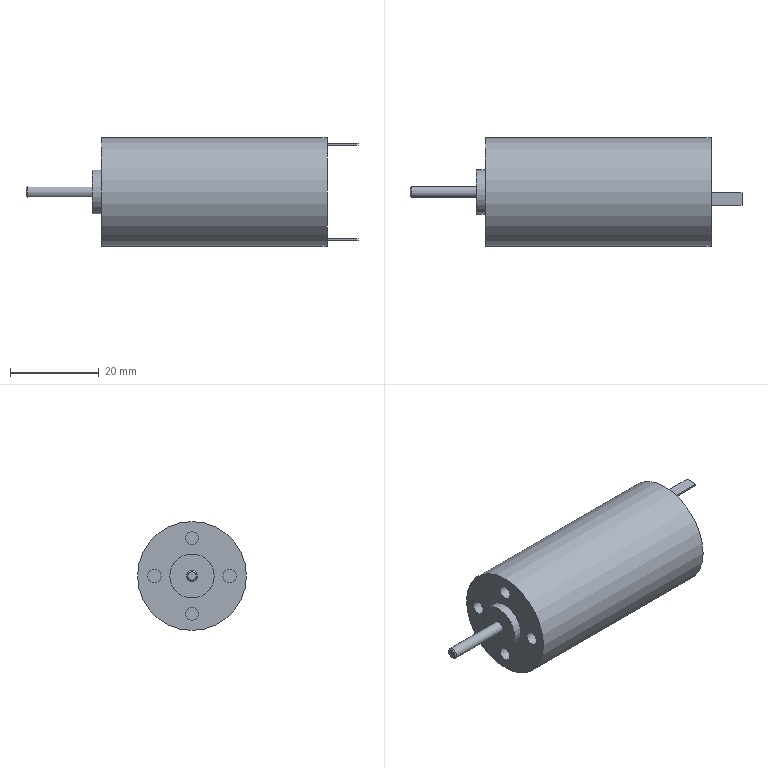Part | STEP file | Wytnij-wyci_gni_cie1_4 | 1 solid | 26 faces | box 75 x 24.6 x 24.6 mm | volume 24401 mm3 | plane 18 | cylinder 7 | cone 1 | commonest cylinder face diameters 3 x4 2.5 x1 10 x1 24.6 x1
STEP:
#1=CARTESIAN_POINT('',(0.,0.,0.));
#2=DIRECTION('',(0.,0.,1.));
#3=DIRECTION('',(1.,0.,0.));
#4=AXIS2_PLACEMENT_3D('',#1,#2,#3);
#5=CARTESIAN_POINT('',(-12.682,75.838,-107.798));
#6=VERTEX_POINT('',#5);
#7=CARTESIAN_POINT('',(38.318,75.838,-107.798));
#8=VERTEX_POINT('',#7);
#9=CARTESIAN_POINT('',(-12.682,75.838,-107.798));
#10=DIRECTION('',(1.,0.,0.));
#11=VECTOR('',#10,1.);
#12=LINE('',#9,#11);
#13=CARTESIAN_POINT('',(38.318,88.138,-107.798));
#14=DIRECTION('',(-1.,0.,0.));
#15=DIRECTION('',(0.,-1.,0.));
#16=AXIS2_PLACEMENT_3D('',#13,#14,#15);
#17=CYLINDRICAL_SURFACE('',#16,12.3);
#18=CARTESIAN_POINT('',(0.,51.));
#19=DIRECTION('',(0.,-1.));
#20=VECTOR('',#19,1.);
#21=LINE('',#18,#20);
#22=(GEOMETRIC_REPRESENTATION_CONTEXT(2)PARAMETRIC_REPRESENTATION_CONTEXT()REPRESENTATION_CONTEXT('',''));
#23=DEFINITIONAL_REPRESENTATION('',(#21),#22);
#24=PCURVE('',#17,#23);
#25=CARTESIAN_POINT('',(6.283,51.));
#26=DIRECTION('',(0.,-1.));
#27=VECTOR('',#26,1.);
#28=LINE('',#25,#27);
#29=(GEOMETRIC_REPRESENTATION_CONTEXT(2)PARAMETRIC_REPRESENTATION_CONTEXT()REPRESENTATION_CONTEXT('',''));
#30=DEFINITIONAL_REPRESENTATION('',(#28),#29);
#31=PCURVE('',#17,#30);
#32=SEAM_CURVE('',#12,(#24,#31),.PCURVE_S1.);
#33=EDGE_CURVE('',#6,#8,#32,.T.);
#34=ORIENTED_EDGE('',*,*,#33,.T.);
#35=CARTESIAN_POINT('',(38.318,88.138,-107.798));
#36=DIRECTION('',(-1.,0.,0.));
#37=DIRECTION('',(0.,-1.,0.));
#38=AXIS2_PLACEMENT_3D('',#35,#36,#37);
#39=CIRCLE('',#38,12.3);
#40=CARTESIAN_POINT('',(0.,0.));
#41=DIRECTION('',(1.,0.));
#42=VECTOR('',#41,1.);
#43=LINE('',#40,#42);
#44=(GEOMETRIC_REPRESENTATION_CONTEXT(2)PARAMETRIC_REPRESENTATION_CONTEXT()REPRESENTATION_CONTEXT('',''));
#45=DEFINITIONAL_REPRESENTATION('',(#43),#44);
#46=PCURVE('',#17,#45);
#47=CARTESIAN_POINT('',(38.318,88.138,-107.798));
#48=DIRECTION('',(1.,0.,0.));
#49=DIRECTION('',(0.,1.,0.));
#50=AXIS2_PLACEMENT_3D('',#47,#48,#49);
#51=PLANE('',#50);
#52=CARTESIAN_POINT('',(-12.3,0.));
#53=CARTESIAN_POINT('',(-12.3,21.304));
#54=CARTESIAN_POINT('',(6.15,10.652));
#55=CARTESIAN_POINT('',(24.6,0.));
#56=CARTESIAN_POINT('',(6.15,-10.652));
#57=CARTESIAN_POINT('',(-12.3,-21.304));
#58=CARTESIAN_POINT('',(-12.3,0.));
#59=(BOUNDED_CURVE()B_SPLINE_CURVE(2,(#52,#53,#54,#55,#56,#57,#58),.UNSPECIFIED.,.T.,.F.)B_SPLINE_CURVE_WITH_KNOTS((1,2,2,2,2,1),(-2.094,0.,2.094,4.189,6.283,8.378),.UNSPECIFIED.)CURVE()GEOMETRIC_REPRESENTATION_ITEM()RATIONAL_B_SPLINE_CURVE((1.,0.5,1.,0.5,1.,0.5,1.))REPRESENTATION_ITEM(''));
#60=(GEOMETRIC_REPRESENTATION_CONTEXT(2)PARAMETRIC_REPRESENTATION_CONTEXT()REPRESENTATION_CONTEXT('',''));
#61=DEFINITIONAL_REPRESENTATION('',(#59),#60);
#62=PCURVE('',#51,#61);
#63=SURFACE_CURVE('',#39,(#46,#62),.PCURVE_S1.);
#64=EDGE_CURVE('',#8,#8,#63,.T.);
#65=ORIENTED_EDGE('',*,*,#64,.T.);
#66=ORIENTED_EDGE('',*,*,#33,.F.);
#67=CARTESIAN_POINT('',(-12.682,88.138,-107.798));
#68=DIRECTION('',(1.,0.,0.));
#69=DIRECTION('',(0.,-1.,0.));
#70=AXIS2_PLACEMENT_3D('',#67,#68,#69);
#71=CIRCLE('',#70,12.3);
#72=CARTESIAN_POINT('',(6.283,51.));
#73=DIRECTION('',(-1.,0.));
#74=VECTOR('',#73,1.);
#75=LINE('',#72,#74);
#76=(GEOMETRIC_REPRESENTATION_CONTEXT(2)PARAMETRIC_REPRESENTATION_CONTEXT()REPRESENTATION_CONTEXT('',''));
#77=DEFINITIONAL_REPRESENTATION('',(#75),#76);
#78=PCURVE('',#17,#77);
#79=CARTESIAN_POINT('',(-12.682,88.138,-107.798));
#80=DIRECTION('',(-1.,0.,0.));
#81=DIRECTION('',(0.,-1.,0.));
#82=AXIS2_PLACEMENT_3D('',#79,#80,#81);
#83=PLANE('',#82);
#84=CARTESIAN_POINT('',(12.3,0.));
#85=CARTESIAN_POINT('',(12.3,-21.304));
#86=CARTESIAN_POINT('',(-6.15,-10.652));
#87=CARTESIAN_POINT('',(-24.6,0.));
#88=CARTESIAN_POINT('',(-6.15,10.652));
#89=CARTESIAN_POINT('',(12.3,21.304));
#90=CARTESIAN_POINT('',(12.3,0.));
#91=(BOUNDED_CURVE()B_SPLINE_CURVE(2,(#84,#85,#86,#87,#88,#89,#90),.UNSPECIFIED.,.T.,.F.)B_SPLINE_CURVE_WITH_KNOTS((1,2,2,2,2,1),(-2.094,0.,2.094,4.189,6.283,8.378),.UNSPECIFIED.)CURVE()GEOMETRIC_REPRESENTATION_ITEM()RATIONAL_B_SPLINE_CURVE((1.,0.5,1.,0.5,1.,0.5,1.))REPRESENTATION_ITEM(''));
#92=(GEOMETRIC_REPRESENTATION_CONTEXT(2)PARAMETRIC_REPRESENTATION_CONTEXT()REPRESENTATION_CONTEXT('',''));
#93=DEFINITIONAL_REPRESENTATION('',(#91),#92);
#94=PCURVE('',#83,#93);
#95=SURFACE_CURVE('',#71,(#78,#94),.PCURVE_S1.);
#96=EDGE_CURVE('',#6,#6,#95,.T.);
#97=ORIENTED_EDGE('',*,*,#96,.T.);
#98=EDGE_LOOP('',(#34,#65,#66,#97));
#99=FACE_BOUND('',#98,.T.);
#100=ADVANCED_FACE('',(#99),#17,.T.);
#101=CARTESIAN_POINT('',(-9.682,86.638,-99.298));
#102=VERTEX_POINT('',#101);
#103=CARTESIAN_POINT('',(-9.682,88.138,-99.298));
#104=DIRECTION('',(-1.,0.,0.));
#105=DIRECTION('',(0.,-1.,0.));
#106=AXIS2_PLACEMENT_3D('',#103,#104,#105);
#107=CIRCLE('',#106,1.5);
#108=CARTESIAN_POINT('',(-9.682,88.138,-99.298));
#109=DIRECTION('',(-1.,0.,0.));
#110=DIRECTION('',(0.,-1.,0.));
#111=AXIS2_PLACEMENT_3D('',#108,#109,#110);
#112=CYLINDRICAL_SURFACE('',#111,1.5);
#113=CARTESIAN_POINT('',(0.,0.));
#114=DIRECTION('',(1.,0.));
#115=VECTOR('',#114,1.);
#116=LINE('',#113,#115);
#117=(GEOMETRIC_REPRESENTATION_CONTEXT(2)PARAMETRIC_REPRESENTATION_CONTEXT()REPRESENTATION_CONTEXT('',''));
#118=DEFINITIONAL_REPRESENTATION('',(#116),#117);
#119=PCURVE('',#112,#118);
#120=CARTESIAN_POINT('',(-9.682,88.138,-99.298));
#121=DIRECTION('',(-1.,0.,0.));
#122=DIRECTION('',(0.,-1.,0.));
#123=AXIS2_PLACEMENT_3D('',#120,#121,#122);
#124=PLANE('',#123);
#125=CARTESIAN_POINT('',(0.,0.));
#126=DIRECTION('',(1.,0.));
#127=AXIS2_PLACEMENT_2D('',#125,#126);
#128=CIRCLE('',#127,1.5);
#129=(GEOMETRIC_REPRESENTATION_CONTEXT(2)PARAMETRIC_REPRESENTATION_CONTEXT()REPRESENTATION_CONTEXT('',''));
#130=DEFINITIONAL_REPRESENTATION('',(#128),#129);
#131=PCURVE('',#124,#130);
#132=SURFACE_CURVE('',#107,(#119,#131),.PCURVE_S1.);
#133=EDGE_CURVE('',#102,#102,#132,.T.);
#134=ORIENTED_EDGE('',*,*,#133,.T.);
#135=CARTESIAN_POINT('',(-12.682,86.638,-99.298));
#136=VERTEX_POINT('',#135);
#137=CARTESIAN_POINT('',(-12.682,86.638,-99.298));
#138=DIRECTION('',(1.,0.,0.));
#139=VECTOR('',#138,1.);
#140=LINE('',#137,#139);
#141=CARTESIAN_POINT('',(6.283,3.));
#142=DIRECTION('',(0.,-1.));
#143=VECTOR('',#142,1.);
#144=LINE('',#141,#143);
#145=(GEOMETRIC_REPRESENTATION_CONTEXT(2)PARAMETRIC_REPRESENTATION_CONTEXT()REPRESENTATION_CONTEXT('',''));
#146=DEFINITIONAL_REPRESENTATION('',(#144),#145);
#147=PCURVE('',#112,#146);
#148=CARTESIAN_POINT('',(0.,3.));
#149=DIRECTION('',(0.,-1.));
#150=VECTOR('',#149,1.);
#151=LINE('',#148,#150);
#152=(GEOMETRIC_REPRESENTATION_CONTEXT(2)PARAMETRIC_REPRESENTATION_CONTEXT()REPRESENTATION_CONTEXT('',''));
#153=DEFINITIONAL_REPRESENTATION('',(#151),#152);
#154=PCURVE('',#112,#153);
#155=SEAM_CURVE('',#140,(#147,#154),.PCURVE_S1.);
#156=EDGE_CURVE('',#136,#102,#155,.T.);
#157=ORIENTED_EDGE('',*,*,#156,.F.);
#158=CARTESIAN_POINT('',(-12.682,88.138,-99.298));
#159=DIRECTION('',(1.,0.,0.));
#160=DIRECTION('',(0.,-1.,0.));
#161=AXIS2_PLACEMENT_3D('',#158,#159,#160);
#162=CIRCLE('',#161,1.5);
#163=CARTESIAN_POINT('',(6.283,3.));
#164=DIRECTION('',(-1.,0.));
#165=VECTOR('',#164,1.);
#166=LINE('',#163,#165);
#167=(GEOMETRIC_REPRESENTATION_CONTEXT(2)PARAMETRIC_REPRESENTATION_CONTEXT()REPRESENTATION_CONTEXT('',''));
#168=DEFINITIONAL_REPRESENTATION('',(#166),#167);
#169=PCURVE('',#112,#168);
#170=CARTESIAN_POINT('',(1.5,8.5));
#171=CARTESIAN_POINT('',(1.5,5.902));
#172=CARTESIAN_POINT('',(-0.75,7.201));
#173=CARTESIAN_POINT('',(-3.,8.5));
#174=CARTESIAN_POINT('',(-0.75,9.799));
#175=CARTESIAN_POINT('',(1.5,11.098));
#176=CARTESIAN_POINT('',(1.5,8.5));
#177=(BOUNDED_CURVE()B_SPLINE_CURVE(2,(#170,#171,#172,#173,#174,#175,#176),.UNSPECIFIED.,.T.,.F.)B_SPLINE_CURVE_WITH_KNOTS((1,2,2,2,2,1),(-2.094,0.,2.094,4.189,6.283,8.378),.UNSPECIFIED.)CURVE()GEOMETRIC_REPRESENTATION_ITEM()RATIONAL_B_SPLINE_CURVE((1.,0.5,1.,0.5,1.,0.5,1.))REPRESENTATION_ITEM(''));
#178=(GEOMETRIC_REPRESENTATION_CONTEXT(2)PARAMETRIC_REPRESENTATION_CONTEXT()REPRESENTATION_CONTEXT('',''));
#179=DEFINITIONAL_REPRESENTATION('',(#177),#178);
#180=PCURVE('',#83,#179);
#181=SURFACE_CURVE('',#162,(#169,#180),.PCURVE_S1.);
#182=EDGE_CURVE('',#136,#136,#181,.T.);
#183=ORIENTED_EDGE('',*,*,#182,.T.);
#184=ORIENTED_EDGE('',*,*,#156,.T.);
#185=EDGE_LOOP('',(#134,#157,#183,#184));
#186=FACE_BOUND('',#185,.F.);
#187=ADVANCED_FACE('',(#186),#112,.F.);
#188=CARTESIAN_POINT('',(-9.682,78.138,-107.798));
#189=VERTEX_POINT('',#188);
#190=CARTESIAN_POINT('',(-9.682,79.638,-107.798));
#191=DIRECTION('',(-1.,0.,0.));
#192=DIRECTION('',(0.,-1.,0.));
#193=AXIS2_PLACEMENT_3D('',#190,#191,#192);
#194=CIRCLE('',#193,1.5);
#195=CARTESIAN_POINT('',(-9.682,79.638,-107.798));
#196=DIRECTION('',(-1.,0.,0.));
#197=DIRECTION('',(0.,-1.,0.));
#198=AXIS2_PLACEMENT_3D('',#195,#196,#197);
#199=CYLINDRICAL_SURFACE('',#198,1.5);
#200=CARTESIAN_POINT('',(0.,0.));
#201=DIRECTION('',(1.,0.));
#202=VECTOR('',#201,1.);
#203=LINE('',#200,#202);
#204=(GEOMETRIC_REPRESENTATION_CONTEXT(2)PARAMETRIC_REPRESENTATION_CONTEXT()REPRESENTATION_CONTEXT('',''));
#205=DEFINITIONAL_REPRESENTATION('',(#203),#204);
#206=PCURVE('',#199,#205);
#207=CARTESIAN_POINT('',(-9.682,79.638,-107.798));
#208=DIRECTION('',(-1.,0.,0.));
#209=DIRECTION('',(0.,-1.,0.));
#210=AXIS2_PLACEMENT_3D('',#207,#208,#209);
#211=PLANE('',#210);
#212=CARTESIAN_POINT('',(0.,0.));
#213=DIRECTION('',(1.,0.));
#214=AXIS2_PLACEMENT_2D('',#212,#213);
#215=CIRCLE('',#214,1.5);
#216=(GEOMETRIC_REPRESENTATION_CONTEXT(2)PARAMETRIC_REPRESENTATION_CONTEXT()REPRESENTATION_CONTEXT('',''));
#217=DEFINITIONAL_REPRESENTATION('',(#215),#216);
#218=PCURVE('',#211,#217);
#219=SURFACE_CURVE('',#194,(#206,#218),.PCURVE_S1.);
#220=EDGE_CURVE('',#189,#189,#219,.T.);
#221=ORIENTED_EDGE('',*,*,#220,.T.);
#222=CARTESIAN_POINT('',(-12.682,78.138,-107.798));
#223=VERTEX_POINT('',#222);
#224=CARTESIAN_POINT('',(-12.682,78.138,-107.798));
#225=DIRECTION('',(1.,0.,0.));
#226=VECTOR('',#225,1.);
#227=LINE('',#224,#226);
#228=CARTESIAN_POINT('',(6.283,3.));
#229=DIRECTION('',(0.,-1.));
#230=VECTOR('',#229,1.);
#231=LINE('',#228,#230);
#232=(GEOMETRIC_REPRESENTATION_CONTEXT(2)PARAMETRIC_REPRESENTATION_CONTEXT()REPRESENTATION_CONTEXT('',''));
#233=DEFINITIONAL_REPRESENTATION('',(#231),#232);
#234=PCURVE('',#199,#233);
#235=CARTESIAN_POINT('',(0.,3.));
#236=DIRECTION('',(0.,-1.));
#237=VECTOR('',#236,1.);
#238=LINE('',#235,#237);
#239=(GEOMETRIC_REPRESENTATION_CONTEXT(2)PARAMETRIC_REPRESENTATION_CONTEXT()REPRESENTATION_CONTEXT('',''));
#240=DEFINITIONAL_REPRESENTATION('',(#238),#239);
#241=PCURVE('',#199,#240);
#242=SEAM_CURVE('',#227,(#234,#241),.PCURVE_S1.);
#243=EDGE_CURVE('',#223,#189,#242,.T.);
#244=ORIENTED_EDGE('',*,*,#243,.F.);
#245=CARTESIAN_POINT('',(-12.682,79.638,-107.798));
#246=DIRECTION('',(1.,0.,0.));
#247=DIRECTION('',(0.,-1.,0.));
#248=AXIS2_PLACEMENT_3D('',#245,#246,#247);
#249=CIRCLE('',#248,1.5);
#250=CARTESIAN_POINT('',(6.283,3.));
#251=DIRECTION('',(-1.,0.));
#252=VECTOR('',#251,1.);
#253=LINE('',#250,#252);
#254=(GEOMETRIC_REPRESENTATION_CONTEXT(2)PARAMETRIC_REPRESENTATION_CONTEXT()REPRESENTATION_CONTEXT('',''));
#255=DEFINITIONAL_REPRESENTATION('',(#253),#254);
#256=PCURVE('',#199,#255);
#257=CARTESIAN_POINT('',(10.,0.));
#258=CARTESIAN_POINT('',(10.,-2.598));
#259=CARTESIAN_POINT('',(7.75,-1.299));
#260=CARTESIAN_POINT('',(5.5,0.));
#261=CARTESIAN_POINT('',(7.75,1.299));
#262=CARTESIAN_POINT('',(10.,2.598));
#263=CARTESIAN_POINT('',(10.,0.));
#264=(BOUNDED_CURVE()B_SPLINE_CURVE(2,(#257,#258,#259,#260,#261,#262,#263),.UNSPECIFIED.,.T.,.F.)B_SPLINE_CURVE_WITH_KNOTS((1,2,2,2,2,1),(-2.094,0.,2.094,4.189,6.283,8.378),.UNSPECIFIED.)CURVE()GEOMETRIC_REPRESENTATION_ITEM()RATIONAL_B_SPLINE_CURVE((1.,0.5,1.,0.5,1.,0.5,1.))REPRESENTATION_ITEM(''));
#265=(GEOMETRIC_REPRESENTATION_CONTEXT(2)PARAMETRIC_REPRESENTATION_CONTEXT()REPRESENTATION_CONTEXT('',''));
#266=DEFINITIONAL_REPRESENTATION('',(#264),#265);
#267=PCURVE('',#83,#266);
#268=SURFACE_CURVE('',#249,(#256,#267),.PCURVE_S1.);
#269=EDGE_CURVE('',#223,#223,#268,.T.);
#270=ORIENTED_EDGE('',*,*,#269,.T.);
#271=ORIENTED_EDGE('',*,*,#243,.T.);
#272=EDGE_LOOP('',(#221,#244,#270,#271));
#273=FACE_BOUND('',#272,.F.);
#274=ADVANCED_FACE('',(#273),#199,.F.);
#275=CARTESIAN_POINT('',(-9.682,86.638,-116.298));
#276=VERTEX_POINT('',#275);
#277=CARTESIAN_POINT('',(-9.682,88.138,-116.298));
#278=DIRECTION('',(-1.,0.,0.));
#279=DIRECTION('',(0.,-1.,0.));
#280=AXIS2_PLACEMENT_3D('',#277,#278,#279);
#281=CIRCLE('',#280,1.5);
#282=CARTESIAN_POINT('',(-9.682,88.138,-116.298));
#283=DIRECTION('',(-1.,0.,0.));
#284=DIRECTION('',(0.,-1.,0.));
#285=AXIS2_PLACEMENT_3D('',#282,#283,#284);
#286=CYLINDRICAL_SURFACE('',#285,1.5);
#287=CARTESIAN_POINT('',(0.,0.));
#288=DIRECTION('',(1.,0.));
#289=VECTOR('',#288,1.);
#290=LINE('',#287,#289);
#291=(GEOMETRIC_REPRESENTATION_CONTEXT(2)PARAMETRIC_REPRESENTATION_CONTEXT()REPRESENTATION_CONTEXT('',''));
#292=DEFINITIONAL_REPRESENTATION('',(#290),#291);
#293=PCURVE('',#286,#292);
#294=CARTESIAN_POINT('',(-9.682,88.138,-116.298));
#295=DIRECTION('',(-1.,0.,0.));
#296=DIRECTION('',(0.,-1.,0.));
#297=AXIS2_PLACEMENT_3D('',#294,#295,#296);
#298=PLANE('',#297);
#299=CARTESIAN_POINT('',(0.,0.));
#300=DIRECTION('',(1.,0.));
#301=AXIS2_PLACEMENT_2D('',#299,#300);
#302=CIRCLE('',#301,1.5);
#303=(GEOMETRIC_REPRESENTATION_CONTEXT(2)PARAMETRIC_REPRESENTATION_CONTEXT()REPRESENTATION_CONTEXT('',''));
#304=DEFINITIONAL_REPRESENTATION('',(#302),#303);
#305=PCURVE('',#298,#304);
#306=SURFACE_CURVE('',#281,(#293,#305),.PCURVE_S1.);
#307=EDGE_CURVE('',#276,#276,#306,.T.);
#308=ORIENTED_EDGE('',*,*,#307,.T.);
#309=CARTESIAN_POINT('',(-12.682,86.638,-116.298));
#310=VERTEX_POINT('',#309);
#311=CARTESIAN_POINT('',(-12.682,86.638,-116.298));
#312=DIRECTION('',(1.,0.,0.));
#313=VECTOR('',#312,1.);
#314=LINE('',#311,#313);
#315=CARTESIAN_POINT('',(6.283,3.));
#316=DIRECTION('',(0.,-1.));
#317=VECTOR('',#316,1.);
#318=LINE('',#315,#317);
#319=(GEOMETRIC_REPRESENTATION_CONTEXT(2)PARAMETRIC_REPRESENTATION_CONTEXT()REPRESENTATION_CONTEXT('',''));
#320=DEFINITIONAL_REPRESENTATION('',(#318),#319);
#321=PCURVE('',#286,#320);
#322=CARTESIAN_POINT('',(0.,3.));
#323=DIRECTION('',(0.,-1.));
#324=VECTOR('',#323,1.);
#325=LINE('',#322,#324);
#326=(GEOMETRIC_REPRESENTATION_CONTEXT(2)PARAMETRIC_REPRESENTATION_CONTEXT()REPRESENTATION_CONTEXT('',''));
#327=DEFINITIONAL_REPRESENTATION('',(#325),#326);
#328=PCURVE('',#286,#327);
#329=SEAM_CURVE('',#314,(#321,#328),.PCURVE_S1.);
#330=EDGE_CURVE('',#310,#276,#329,.T.);
#331=ORIENTED_EDGE('',*,*,#330,.F.);
#332=CARTESIAN_POINT('',(-12.682,88.138,-116.298));
#333=DIRECTION('',(1.,0.,0.));
#334=DIRECTION('',(0.,-1.,0.));
#335=AXIS2_PLACEMENT_3D('',#332,#333,#334);
#336=CIRCLE('',#335,1.5);
#337=CARTESIAN_POINT('',(6.283,3.));
#338=DIRECTION('',(-1.,0.));
#339=VECTOR('',#338,1.);
#340=LINE('',#337,#339);
#341=(GEOMETRIC_REPRESENTATION_CONTEXT(2)PARAMETRIC_REPRESENTATION_CONTEXT()REPRESENTATION_CONTEXT('',''));
#342=DEFINITIONAL_REPRESENTATION('',(#340),#341);
#343=PCURVE('',#286,#342);
#344=CARTESIAN_POINT('',(1.5,-8.5));
#345=CARTESIAN_POINT('',(1.5,-11.098));
#346=CARTESIAN_POINT('',(-0.75,-9.799));
#347=CARTESIAN_POINT('',(-3.,-8.5));
#348=CARTESIAN_POINT('',(-0.75,-7.201));
#349=CARTESIAN_POINT('',(1.5,-5.902));
#350=CARTESIAN_POINT('',(1.5,-8.5));
#351=(BOUNDED_CURVE()B_SPLINE_CURVE(2,(#344,#345,#346,#347,#348,#349,#350),.UNSPECIFIED.,.T.,.F.)B_SPLINE_CURVE_WITH_KNOTS((1,2,2,2,2,1),(-2.094,0.,2.094,4.189,6.283,8.378),.UNSPECIFIED.)CURVE()GEOMETRIC_REPRESENTATION_ITEM()RATIONAL_B_SPLINE_CURVE((1.,0.5,1.,0.5,1.,0.5,1.))REPRESENTATION_ITEM(''));
#352=(GEOMETRIC_REPRESENTATION_CONTEXT(2)PARAMETRIC_REPRESENTATION_CONTEXT()REPRESENTATION_CONTEXT('',''));
#353=DEFINITIONAL_REPRESENTATION('',(#351),#352);
#354=PCURVE('',#83,#353);
#355=SURFACE_CURVE('',#336,(#343,#354),.PCURVE_S1.);
#356=EDGE_CURVE('',#310,#310,#355,.T.);
#357=ORIENTED_EDGE('',*,*,#356,.T.);
#358=ORIENTED_EDGE('',*,*,#330,.T.);
#359=EDGE_LOOP('',(#308,#331,#357,#358));
#360=FACE_BOUND('',#359,.F.);
#361=ADVANCED_FACE('',(#360),#286,.F.);
#362=CARTESIAN_POINT('',(-9.682,95.138,-107.798));
#363=VERTEX_POINT('',#362);
#364=CARTESIAN_POINT('',(-9.682,96.638,-107.798));
#365=DIRECTION('',(-1.,0.,0.));
#366=DIRECTION('',(0.,-1.,0.));
#367=AXIS2_PLACEMENT_3D('',#364,#365,#366);
#368=CIRCLE('',#367,1.5);
#369=CARTESIAN_POINT('',(-9.682,96.638,-107.798));
#370=DIRECTION('',(-1.,0.,0.));
#371=DIRECTION('',(0.,-1.,0.));
#372=AXIS2_PLACEMENT_3D('',#369,#370,#371);
#373=CYLINDRICAL_SURFACE('',#372,1.5);
#374=CARTESIAN_POINT('',(0.,0.));
#375=DIRECTION('',(1.,0.));
#376=VECTOR('',#375,1.);
#377=LINE('',#374,#376);
#378=(GEOMETRIC_REPRESENTATION_CONTEXT(2)PARAMETRIC_REPRESENTATION_CONTEXT()REPRESENTATION_CONTEXT('',''));
#379=DEFINITIONAL_REPRESENTATION('',(#377),#378);
#380=PCURVE('',#373,#379);
#381=CARTESIAN_POINT('',(-9.682,96.638,-107.798));
#382=DIRECTION('',(-1.,0.,0.));
#383=DIRECTION('',(0.,-1.,0.));
#384=AXIS2_PLACEMENT_3D('',#381,#382,#383);
#385=PLANE('',#384);
#386=CARTESIAN_POINT('',(0.,0.));
#387=DIRECTION('',(1.,0.));
#388=AXIS2_PLACEMENT_2D('',#386,#387);
#389=CIRCLE('',#388,1.5);
#390=(GEOMETRIC_REPRESENTATION_CONTEXT(2)PARAMETRIC_REPRESENTATION_CONTEXT()REPRESENTATION_CONTEXT('',''));
#391=DEFINITIONAL_REPRESENTATION('',(#389),#390);
#392=PCURVE('',#385,#391);
#393=SURFACE_CURVE('',#368,(#380,#392),.PCURVE_S1.);
#394=EDGE_CURVE('',#363,#363,#393,.T.);
#395=ORIENTED_EDGE('',*,*,#394,.T.);
#396=CARTESIAN_POINT('',(-12.682,95.138,-107.798));
#397=VERTEX_POINT('',#396);
#398=CARTESIAN_POINT('',(-12.682,95.138,-107.798));
#399=DIRECTION('',(1.,0.,0.));
#400=VECTOR('',#399,1.);
#401=LINE('',#398,#400);
#402=CARTESIAN_POINT('',(6.283,3.));
#403=DIRECTION('',(0.,-1.));
#404=VECTOR('',#403,1.);
#405=LINE('',#402,#404);
#406=(GEOMETRIC_REPRESENTATION_CONTEXT(2)PARAMETRIC_REPRESENTATION_CONTEXT()REPRESENTATION_CONTEXT('',''));
#407=DEFINITIONAL_REPRESENTATION('',(#405),#406);
#408=PCURVE('',#373,#407);
#409=CARTESIAN_POINT('',(0.,3.));
#410=DIRECTION('',(0.,-1.));
#411=VECTOR('',#410,1.);
#412=LINE('',#409,#411);
#413=(GEOMETRIC_REPRESENTATION_CONTEXT(2)PARAMETRIC_REPRESENTATION_CONTEXT()REPRESENTATION_CONTEXT('',''));
#414=DEFINITIONAL_REPRESENTATION('',(#412),#413);
#415=PCURVE('',#373,#414);
#416=SEAM_CURVE('',#401,(#408,#415),.PCURVE_S1.);
#417=EDGE_CURVE('',#397,#363,#416,.T.);
#418=ORIENTED_EDGE('',*,*,#417,.F.);
#419=CARTESIAN_POINT('',(-12.682,96.638,-107.798));
#420=DIRECTION('',(1.,0.,0.));
#421=DIRECTION('',(0.,-1.,0.));
#422=AXIS2_PLACEMENT_3D('',#419,#420,#421);
#423=CIRCLE('',#422,1.5);
#424=CARTESIAN_POINT('',(6.283,3.));
#425=DIRECTION('',(-1.,0.));
#426=VECTOR('',#425,1.);
#427=LINE('',#424,#426);
#428=(GEOMETRIC_REPRESENTATION_CONTEXT(2)PARAMETRIC_REPRESENTATION_CONTEXT()REPRESENTATION_CONTEXT('',''));
#429=DEFINITIONAL_REPRESENTATION('',(#427),#428);
#430=PCURVE('',#373,#429);
#431=CARTESIAN_POINT('',(-7.,0.));
#432=CARTESIAN_POINT('',(-7.,-2.598));
#433=CARTESIAN_POINT('',(-9.25,-1.299));
#434=CARTESIAN_POINT('',(-11.5,0.));
#435=CARTESIAN_POINT('',(-9.25,1.299));
#436=CARTESIAN_POINT('',(-7.,2.598));
#437=CARTESIAN_POINT('',(-7.,0.));
#438=(BOUNDED_CURVE()B_SPLINE_CURVE(2,(#431,#432,#433,#434,#435,#436,#437),.UNSPECIFIED.,.T.,.F.)B_SPLINE_CURVE_WITH_KNOTS((1,2,2,2,2,1),(-2.094,0.,2.094,4.189,6.283,8.378),.UNSPECIFIED.)CURVE()GEOMETRIC_REPRESENTATION_ITEM()RATIONAL_B_SPLINE_CURVE((1.,0.5,1.,0.5,1.,0.5,1.))REPRESENTATION_ITEM(''));
#439=(GEOMETRIC_REPRESENTATION_CONTEXT(2)PARAMETRIC_REPRESENTATION_CONTEXT()REPRESENTATION_CONTEXT('',''));
#440=DEFINITIONAL_REPRESENTATION('',(#438),#439);
#441=PCURVE('',#83,#440);
#442=SURFACE_CURVE('',#423,(#430,#441),.PCURVE_S1.);
#443=EDGE_CURVE('',#397,#397,#442,.T.);
#444=ORIENTED_EDGE('',*,*,#443,.T.);
#445=ORIENTED_EDGE('',*,*,#417,.T.);
#446=EDGE_LOOP('',(#395,#418,#444,#445));
#447=FACE_BOUND('',#446,.F.);
#448=ADVANCED_FACE('',(#447),#373,.F.);
#449=CARTESIAN_POINT('',(-12.682,93.138,-107.798));
#450=VERTEX_POINT('',#449);
#451=CARTESIAN_POINT('',(-14.682,93.138,-107.798));
#452=VERTEX_POINT('',#451);
#453=CARTESIAN_POINT('',(-12.682,93.138,-107.798));
#454=DIRECTION('',(-1.,0.,0.));
#455=VECTOR('',#454,1.);
#456=LINE('',#453,#455);
#457=CARTESIAN_POINT('',(-14.682,88.138,-107.798));
#458=DIRECTION('',(1.,0.,0.));
#459=DIRECTION('',(0.,1.,0.));
#460=AXIS2_PLACEMENT_3D('',#457,#458,#459);
#461=CYLINDRICAL_SURFACE('',#460,5.);
#462=CARTESIAN_POINT('',(0.,2.));
#463=DIRECTION('',(0.,-1.));
#464=VECTOR('',#463,1.);
#465=LINE('',#462,#464);
#466=(GEOMETRIC_REPRESENTATION_CONTEXT(2)PARAMETRIC_REPRESENTATION_CONTEXT()REPRESENTATION_CONTEXT('',''));
#467=DEFINITIONAL_REPRESENTATION('',(#465),#466);
#468=PCURVE('',#461,#467);
#469=CARTESIAN_POINT('',(6.283,2.));
#470=DIRECTION('',(0.,-1.));
#471=VECTOR('',#470,1.);
#472=LINE('',#469,#471);
#473=(GEOMETRIC_REPRESENTATION_CONTEXT(2)PARAMETRIC_REPRESENTATION_CONTEXT()REPRESENTATION_CONTEXT('',''));
#474=DEFINITIONAL_REPRESENTATION('',(#472),#473);
#475=PCURVE('',#461,#474);
#476=SEAM_CURVE('',#456,(#468,#475),.PCURVE_S1.);
#477=EDGE_CURVE('',#450,#452,#476,.T.);
#478=ORIENTED_EDGE('',*,*,#477,.T.);
#479=CARTESIAN_POINT('',(-14.682,88.138,-107.798));
#480=DIRECTION('',(1.,0.,0.));
#481=DIRECTION('',(0.,1.,0.));
#482=AXIS2_PLACEMENT_3D('',#479,#480,#481);
#483=CIRCLE('',#482,5.);
#484=CARTESIAN_POINT('',(0.,0.));
#485=DIRECTION('',(1.,0.));
#486=VECTOR('',#485,1.);
#487=LINE('',#484,#486);
#488=(GEOMETRIC_REPRESENTATION_CONTEXT(2)PARAMETRIC_REPRESENTATION_CONTEXT()REPRESENTATION_CONTEXT('',''));
#489=DEFINITIONAL_REPRESENTATION('',(#487),#488);
#490=PCURVE('',#461,#489);
#491=CARTESIAN_POINT('',(-14.682,88.138,-107.798));
#492=DIRECTION('',(-1.,0.,0.));
#493=DIRECTION('',(0.,-1.,0.));
#494=AXIS2_PLACEMENT_3D('',#491,#492,#493);
#495=PLANE('',#494);
#496=CARTESIAN_POINT('',(-5.,0.));
#497=CARTESIAN_POINT('',(-5.,8.66));
#498=CARTESIAN_POINT('',(2.5,4.33));
#499=CARTESIAN_POINT('',(10.,0.));
#500=CARTESIAN_POINT('',(2.5,-4.33));
#501=CARTESIAN_POINT('',(-5.,-8.66));
#502=CARTESIAN_POINT('',(-5.,0.));
#503=(BOUNDED_CURVE()B_SPLINE_CURVE(2,(#496,#497,#498,#499,#500,#501,#502),.UNSPECIFIED.,.T.,.F.)B_SPLINE_CURVE_WITH_KNOTS((1,2,2,2,2,1),(-2.094,0.,2.094,4.189,6.283,8.378),.UNSPECIFIED.)CURVE()GEOMETRIC_REPRESENTATION_ITEM()RATIONAL_B_SPLINE_CURVE((1.,0.5,1.,0.5,1.,0.5,1.))REPRESENTATION_ITEM(''));
#504=(GEOMETRIC_REPRESENTATION_CONTEXT(2)PARAMETRIC_REPRESENTATION_CONTEXT()REPRESENTATION_CONTEXT('',''));
#505=DEFINITIONAL_REPRESENTATION('',(#503),#504);
#506=PCURVE('',#495,#505);
#507=SURFACE_CURVE('',#483,(#490,#506),.PCURVE_S1.);
#508=EDGE_CURVE('',#452,#452,#507,.T.);
#509=ORIENTED_EDGE('',*,*,#508,.T.);
#510=ORIENTED_EDGE('',*,*,#477,.F.);
#511=CARTESIAN_POINT('',(-12.682,88.138,-107.798));
#512=DIRECTION('',(1.,0.,0.));
#513=DIRECTION('',(0.,1.,0.));
#514=AXIS2_PLACEMENT_3D('',#511,#512,#513);
#515=CIRCLE('',#514,5.);
#516=CARTESIAN_POINT('',(0.,2.));
#517=DIRECTION('',(1.,0.));
#518=VECTOR('',#517,1.);
#519=LINE('',#516,#518);
#520=(GEOMETRIC_REPRESENTATION_CONTEXT(2)PARAMETRIC_REPRESENTATION_CONTEXT()REPRESENTATION_CONTEXT('',''));
#521=DEFINITIONAL_REPRESENTATION('',(#519),#520);
#522=PCURVE('',#461,#521);
#523=CARTESIAN_POINT('',(-5.,0.));
#524=CARTESIAN_POINT('',(-5.,8.66));
#525=CARTESIAN_POINT('',(2.5,4.33));
#526=CARTESIAN_POINT('',(10.,0.));
#527=CARTESIAN_POINT('',(2.5,-4.33));
#528=CARTESIAN_POINT('',(-5.,-8.66));
#529=CARTESIAN_POINT('',(-5.,0.));
#530=(BOUNDED_CURVE()B_SPLINE_CURVE(2,(#523,#524,#525,#526,#527,#528,#529),.UNSPECIFIED.,.T.,.F.)B_SPLINE_CURVE_WITH_KNOTS((1,2,2,2,2,1),(-2.094,0.,2.094,4.189,6.283,8.378),.UNSPECIFIED.)CURVE()GEOMETRIC_REPRESENTATION_ITEM()RATIONAL_B_SPLINE_CURVE((1.,0.5,1.,0.5,1.,0.5,1.))REPRESENTATION_ITEM(''));
#531=(GEOMETRIC_REPRESENTATION_CONTEXT(2)PARAMETRIC_REPRESENTATION_CONTEXT()REPRESENTATION_CONTEXT('',''));
#532=DEFINITIONAL_REPRESENTATION('',(#530),#531);
#533=PCURVE('',#83,#532);
#534=SURFACE_CURVE('',#515,(#522,#533),.PCURVE_S1.);
#535=EDGE_CURVE('',#450,#450,#534,.T.);
#536=ORIENTED_EDGE('',*,*,#535,.F.);
#537=EDGE_LOOP('',(#478,#509,#510,#536));
#538=FACE_BOUND('',#537,.T.);
#539=ADVANCED_FACE('',(#538),#461,.T.);
#540=CARTESIAN_POINT('',(-14.682,89.388,-107.798));
#541=VERTEX_POINT('',#540);
#542=CARTESIAN_POINT('',(-29.382,89.388,-107.798));
#543=VERTEX_POINT('',#542);
#544=CARTESIAN_POINT('',(-14.682,89.388,-107.798));
#545=DIRECTION('',(-1.,0.,0.));
#546=VECTOR('',#545,1.);
#547=LINE('',#544,#546);
#548=CARTESIAN_POINT('',(-29.382,88.138,-107.798));
#549=DIRECTION('',(1.,0.,0.));
#550=DIRECTION('',(0.,1.,0.));
#551=AXIS2_PLACEMENT_3D('',#548,#549,#550);
#552=CYLINDRICAL_SURFACE('',#551,1.25);
#553=CARTESIAN_POINT('',(0.,14.7));
#554=DIRECTION('',(0.,-1.));
#555=VECTOR('',#554,1.);
#556=LINE('',#553,#555);
#557=(GEOMETRIC_REPRESENTATION_CONTEXT(2)PARAMETRIC_REPRESENTATION_CONTEXT()REPRESENTATION_CONTEXT('',''));
#558=DEFINITIONAL_REPRESENTATION('',(#556),#557);
#559=PCURVE('',#552,#558);
#560=CARTESIAN_POINT('',(6.283,14.7));
#561=DIRECTION('',(0.,-1.));
#562=VECTOR('',#561,1.);
#563=LINE('',#560,#562);
#564=(GEOMETRIC_REPRESENTATION_CONTEXT(2)PARAMETRIC_REPRESENTATION_CONTEXT()REPRESENTATION_CONTEXT('',''));
#565=DEFINITIONAL_REPRESENTATION('',(#563),#564);
#566=PCURVE('',#552,#565);
#567=SEAM_CURVE('',#547,(#559,#566),.PCURVE_S1.);
#568=EDGE_CURVE('',#541,#543,#567,.T.);
#569=ORIENTED_EDGE('',*,*,#568,.T.);
#570=CARTESIAN_POINT('',(-29.382,88.138,-107.798));
#571=DIRECTION('',(1.,0.,0.));
#572=DIRECTION('',(0.,1.,0.));
#573=AXIS2_PLACEMENT_3D('',#570,#571,#572);
#574=CIRCLE('',#573,1.25);
#575=CARTESIAN_POINT('',(0.,0.));
#576=DIRECTION('',(1.,0.));
#577=VECTOR('',#576,1.);
#578=LINE('',#575,#577);
#579=(GEOMETRIC_REPRESENTATION_CONTEXT(2)PARAMETRIC_REPRESENTATION_CONTEXT()REPRESENTATION_CONTEXT('',''));
#580=DEFINITIONAL_REPRESENTATION('',(#578),#579);
#581=PCURVE('',#552,#580);
#582=CARTESIAN_POINT('',(-29.382,88.138,-107.798));
#583=DIRECTION('',(1.,0.,0.));
#584=DIRECTION('',(0.,1.,0.));
#585=AXIS2_PLACEMENT_3D('',#582,#583,#584);
#586=CONICAL_SURFACE('',#585,1.25,0.7854);
#587=CARTESIAN_POINT('',(0.,0.));
#588=DIRECTION('',(1.,0.));
#589=VECTOR('',#588,1.);
#590=LINE('',#587,#589);
#591=(GEOMETRIC_REPRESENTATION_CONTEXT(2)PARAMETRIC_REPRESENTATION_CONTEXT()REPRESENTATION_CONTEXT('',''));
#592=DEFINITIONAL_REPRESENTATION('',(#590),#591);
#593=PCURVE('',#586,#592);
#594=SURFACE_CURVE('',#574,(#581,#593),.PCURVE_S1.);
#595=EDGE_CURVE('',#543,#543,#594,.T.);
#596=ORIENTED_EDGE('',*,*,#595,.T.);
#597=ORIENTED_EDGE('',*,*,#568,.F.);
#598=CARTESIAN_POINT('',(-14.682,88.138,-107.798));
#599=DIRECTION('',(1.,0.,0.));
#600=DIRECTION('',(0.,1.,0.));
#601=AXIS2_PLACEMENT_3D('',#598,#599,#600);
#602=CIRCLE('',#601,1.25);
#603=CARTESIAN_POINT('',(0.,14.7));
#604=DIRECTION('',(1.,0.));
#605=VECTOR('',#604,1.);
#606=LINE('',#603,#605);
#607=(GEOMETRIC_REPRESENTATION_CONTEXT(2)PARAMETRIC_REPRESENTATION_CONTEXT()REPRESENTATION_CONTEXT('',''));
#608=DEFINITIONAL_REPRESENTATION('',(#606),#607);
#609=PCURVE('',#552,#608);
#610=CARTESIAN_POINT('',(-1.25,0.));
#611=CARTESIAN_POINT('',(-1.25,2.165));
#612=CARTESIAN_POINT('',(0.625,1.083));
#613=CARTESIAN_POINT('',(2.5,0.));
#614=CARTESIAN_POINT('',(0.625,-1.083));
#615=CARTESIAN_POINT('',(-1.25,-2.165));
#616=CARTESIAN_POINT('',(-1.25,0.));
#617=(BOUNDED_CURVE()B_SPLINE_CURVE(2,(#610,#611,#612,#613,#614,#615,#616),.UNSPECIFIED.,.T.,.F.)B_SPLINE_CURVE_WITH_KNOTS((1,2,2,2,2,1),(-2.094,0.,2.094,4.189,6.283,8.378),.UNSPECIFIED.)CURVE()GEOMETRIC_REPRESENTATION_ITEM()RATIONAL_B_SPLINE_CURVE((1.,0.5,1.,0.5,1.,0.5,1.))REPRESENTATION_ITEM(''));
#618=(GEOMETRIC_REPRESENTATION_CONTEXT(2)PARAMETRIC_REPRESENTATION_CONTEXT()REPRESENTATION_CONTEXT('',''));
#619=DEFINITIONAL_REPRESENTATION('',(#617),#618);
#620=PCURVE('',#495,#619);
#621=SURFACE_CURVE('',#602,(#609,#620),.PCURVE_S1.);
#622=EDGE_CURVE('',#541,#541,#621,.T.);
#623=ORIENTED_EDGE('',*,*,#622,.F.);
#624=EDGE_LOOP('',(#569,#596,#597,#623));
#625=FACE_BOUND('',#624,.T.);
#626=ADVANCED_FACE('',(#625),#552,.T.);
#627=CARTESIAN_POINT('',(-29.682,89.088,-107.798));
#628=VERTEX_POINT('',#627);
#629=CARTESIAN_POINT('',(-29.382,89.388,-107.798));
#630=DIRECTION('',(-0.7071,-0.7071,0.));
#631=VECTOR('',#630,1.);
#632=LINE('',#629,#631);
#633=CARTESIAN_POINT('',(0.,0.));
#634=DIRECTION('',(0.,-1.));
#635=VECTOR('',#634,1.);
#636=LINE('',#633,#635);
#637=(GEOMETRIC_REPRESENTATION_CONTEXT(2)PARAMETRIC_REPRESENTATION_CONTEXT()REPRESENTATION_CONTEXT('',''));
#638=DEFINITIONAL_REPRESENTATION('',(#636),#637);
#639=PCURVE('',#586,#638);
#640=CARTESIAN_POINT('',(6.283,0.));
#641=DIRECTION('',(0.,-1.));
#642=VECTOR('',#641,1.);
#643=LINE('',#640,#642);
#644=(GEOMETRIC_REPRESENTATION_CONTEXT(2)PARAMETRIC_REPRESENTATION_CONTEXT()REPRESENTATION_CONTEXT('',''));
#645=DEFINITIONAL_REPRESENTATION('',(#643),#644);
#646=PCURVE('',#586,#645);
#647=SEAM_CURVE('',#632,(#639,#646),.PCURVE_S1.);
#648=EDGE_CURVE('',#543,#628,#647,.T.);
#649=ORIENTED_EDGE('',*,*,#648,.T.);
#650=CARTESIAN_POINT('',(-29.682,88.138,-107.798));
#651=DIRECTION('',(1.,0.,0.));
#652=DIRECTION('',(0.,1.,0.));
#653=AXIS2_PLACEMENT_3D('',#650,#651,#652);
#654=CIRCLE('',#653,0.95);
#655=CARTESIAN_POINT('',(0.,-0.3));
#656=DIRECTION('',(1.,0.));
#657=VECTOR('',#656,1.);
#658=LINE('',#655,#657);
#659=(GEOMETRIC_REPRESENTATION_CONTEXT(2)PARAMETRIC_REPRESENTATION_CONTEXT()REPRESENTATION_CONTEXT('',''));
#660=DEFINITIONAL_REPRESENTATION('',(#658),#659);
#661=PCURVE('',#586,#660);
#662=CARTESIAN_POINT('',(-29.682,88.138,-107.798));
#663=DIRECTION('',(-1.,0.,0.));
#664=DIRECTION('',(0.,-1.,0.));
#665=AXIS2_PLACEMENT_3D('',#662,#663,#664);
#666=PLANE('',#665);
#667=CARTESIAN_POINT('',(-0.95,0.));
#668=CARTESIAN_POINT('',(-0.95,1.645));
#669=CARTESIAN_POINT('',(0.475,0.8227));
#670=CARTESIAN_POINT('',(1.9,0.));
#671=CARTESIAN_POINT('',(0.475,-0.8227));
#672=CARTESIAN_POINT('',(-0.95,-1.645));
#673=CARTESIAN_POINT('',(-0.95,0.));
#674=(BOUNDED_CURVE()B_SPLINE_CURVE(2,(#667,#668,#669,#670,#671,#672,#673),.UNSPECIFIED.,.T.,.F.)B_SPLINE_CURVE_WITH_KNOTS((1,2,2,2,2,1),(-2.094,0.,2.094,4.189,6.283,8.378),.UNSPECIFIED.)CURVE()GEOMETRIC_REPRESENTATION_ITEM()RATIONAL_B_SPLINE_CURVE((1.,0.5,1.,0.5,1.,0.5,1.))REPRESENTATION_ITEM(''));
#675=(GEOMETRIC_REPRESENTATION_CONTEXT(2)PARAMETRIC_REPRESENTATION_CONTEXT()REPRESENTATION_CONTEXT('',''));
#676=DEFINITIONAL_REPRESENTATION('',(#674),#675);
#677=PCURVE('',#666,#676);
#678=SURFACE_CURVE('',#654,(#661,#677),.PCURVE_S1.);
#679=EDGE_CURVE('',#628,#628,#678,.T.);
#680=ORIENTED_EDGE('',*,*,#679,.T.);
#681=ORIENTED_EDGE('',*,*,#648,.F.);
#682=ORIENTED_EDGE('',*,*,#595,.F.);
#683=EDGE_LOOP('',(#649,#680,#681,#682));
#684=FACE_BOUND('',#683,.T.);
#685=ADVANCED_FACE('',(#684),#586,.T.);
#686=ORIENTED_EDGE('',*,*,#182,.T.);
#687=EDGE_LOOP('',(#686));
#688=FACE_BOUND('',#687,.T.);
#689=ORIENTED_EDGE('',*,*,#269,.T.);
#690=EDGE_LOOP('',(#689));
#691=FACE_BOUND('',#690,.T.);
#692=ORIENTED_EDGE('',*,*,#356,.T.);
#693=EDGE_LOOP('',(#692));
#694=FACE_BOUND('',#693,.T.);
#695=ORIENTED_EDGE('',*,*,#443,.T.);
#696=EDGE_LOOP('',(#695));
#697=FACE_BOUND('',#696,.T.);
#698=ORIENTED_EDGE('',*,*,#535,.T.);
#699=EDGE_LOOP('',(#698));
#700=FACE_BOUND('',#699,.T.);
#701=ORIENTED_EDGE('',*,*,#96,.F.);
#702=EDGE_LOOP('',(#701));
#703=FACE_BOUND('',#702,.T.);
#704=ADVANCED_FACE('',(#688,#691,#694,#697,#700,#703),#83,.T.);
#705=CARTESIAN_POINT('',(38.318,85.136,-96.798));
#706=VERTEX_POINT('',#705);
#707=CARTESIAN_POINT('',(38.318,87.936,-96.798));
#708=VERTEX_POINT('',#707);
#709=CARTESIAN_POINT('',(38.318,85.136,-96.798));
#710=DIRECTION('',(0.,1.,0.));
#711=VECTOR('',#710,1.);
#712=LINE('',#709,#711);
#713=CARTESIAN_POINT('',(-3.002,11.));
#714=DIRECTION('',(1.,0.));
#715=VECTOR('',#714,1.);
#716=LINE('',#713,#715);
#717=(GEOMETRIC_REPRESENTATION_CONTEXT(2)PARAMETRIC_REPRESENTATION_CONTEXT()REPRESENTATION_CONTEXT('',''));
#718=DEFINITIONAL_REPRESENTATION('',(#716),#717);
#719=PCURVE('',#51,#718);
#720=CARTESIAN_POINT('',(41.818,86.536,-96.798));
#721=DIRECTION('',(0.,0.,-1.));
#722=DIRECTION('',(-1.,0.,0.));
#723=AXIS2_PLACEMENT_3D('',#720,#721,#722);
#724=PLANE('',#723);
#725=CARTESIAN_POINT('',(3.5,-1.4));
#726=DIRECTION('',(0.,1.));
#727=VECTOR('',#726,1.);
#728=LINE('',#725,#727);
#729=(GEOMETRIC_REPRESENTATION_CONTEXT(2)PARAMETRIC_REPRESENTATION_CONTEXT()REPRESENTATION_CONTEXT('',''));
#730=DEFINITIONAL_REPRESENTATION('',(#728),#729);
#731=PCURVE('',#724,#730);
#732=SURFACE_CURVE('',#712,(#719,#731),.PCURVE_S1.);
#733=EDGE_CURVE('',#706,#708,#732,.T.);
#734=ORIENTED_EDGE('',*,*,#733,.T.);
#735=CARTESIAN_POINT('',(38.318,87.936,-97.198));
#736=VERTEX_POINT('',#735);
#737=CARTESIAN_POINT('',(38.318,87.936,-96.798));
#738=DIRECTION('',(0.,0.,-1.));
#739=VECTOR('',#738,1.);
#740=LINE('',#737,#739);
#741=CARTESIAN_POINT('',(-0.2021,11.));
#742=DIRECTION('',(0.,-1.));
#743=VECTOR('',#742,1.);
#744=LINE('',#741,#743);
#745=(GEOMETRIC_REPRESENTATION_CONTEXT(2)PARAMETRIC_REPRESENTATION_CONTEXT()REPRESENTATION_CONTEXT('',''));
#746=DEFINITIONAL_REPRESENTATION('',(#744),#745);
#747=PCURVE('',#51,#746);
#748=CARTESIAN_POINT('',(41.818,87.936,-96.998));
#749=DIRECTION('',(0.,-1.,0.));
#750=DIRECTION('',(1.,0.,0.));
#751=AXIS2_PLACEMENT_3D('',#748,#749,#750);
#752=PLANE('',#751);
#753=CARTESIAN_POINT('',(-3.5,0.2));
#754=DIRECTION('',(0.,-1.));
#755=VECTOR('',#754,1.);
#756=LINE('',#753,#755);
#757=(GEOMETRIC_REPRESENTATION_CONTEXT(2)PARAMETRIC_REPRESENTATION_CONTEXT()REPRESENTATION_CONTEXT('',''));
#758=DEFINITIONAL_REPRESENTATION('',(#756),#757);
#759=PCURVE('',#752,#758);
#760=SURFACE_CURVE('',#740,(#747,#759),.PCURVE_S1.);
#761=EDGE_CURVE('',#708,#736,#760,.T.);
#762=ORIENTED_EDGE('',*,*,#761,.T.);
#763=CARTESIAN_POINT('',(38.318,85.136,-97.198));
#764=VERTEX_POINT('',#763);
#765=CARTESIAN_POINT('',(38.318,87.936,-97.198));
#766=DIRECTION('',(0.,-1.,0.));
#767=VECTOR('',#766,1.);
#768=LINE('',#765,#767);
#769=CARTESIAN_POINT('',(-0.2021,10.6));
#770=DIRECTION('',(-1.,0.));
#771=VECTOR('',#770,1.);
#772=LINE('',#769,#771);
#773=(GEOMETRIC_REPRESENTATION_CONTEXT(2)PARAMETRIC_REPRESENTATION_CONTEXT()REPRESENTATION_CONTEXT('',''));
#774=DEFINITIONAL_REPRESENTATION('',(#772),#773);
#775=PCURVE('',#51,#774);
#776=CARTESIAN_POINT('',(41.818,86.536,-97.198));
#777=DIRECTION('',(0.,0.,1.));
#778=DIRECTION('',(1.,0.,0.));
#779=AXIS2_PLACEMENT_3D('',#776,#777,#778);
#780=PLANE('',#779);
#781=CARTESIAN_POINT('',(-3.5,1.4));
#782=DIRECTION('',(0.,-1.));
#783=VECTOR('',#782,1.);
#784=LINE('',#781,#783);
#785=(GEOMETRIC_REPRESENTATION_CONTEXT(2)PARAMETRIC_REPRESENTATION_CONTEXT()REPRESENTATION_CONTEXT('',''));
#786=DEFINITIONAL_REPRESENTATION('',(#784),#785);
#787=PCURVE('',#780,#786);
#788=SURFACE_CURVE('',#768,(#775,#787),.PCURVE_S1.);
#789=EDGE_CURVE('',#736,#764,#788,.T.);
#790=ORIENTED_EDGE('',*,*,#789,.T.);
#791=CARTESIAN_POINT('',(38.318,85.136,-97.198));
#792=DIRECTION('',(0.,0.,1.));
#793=VECTOR('',#792,1.);
#794=LINE('',#791,#793);
#795=CARTESIAN_POINT('',(-3.002,10.6));
#796=DIRECTION('',(0.,1.));
#797=VECTOR('',#796,1.);
#798=LINE('',#795,#797);
#799=(GEOMETRIC_REPRESENTATION_CONTEXT(2)PARAMETRIC_REPRESENTATION_CONTEXT()REPRESENTATION_CONTEXT('',''));
#800=DEFINITIONAL_REPRESENTATION('',(#798),#799);
#801=PCURVE('',#51,#800);
#802=CARTESIAN_POINT('',(41.818,85.136,-96.998));
#803=DIRECTION('',(0.,1.,0.));
#804=DIRECTION('',(-1.,0.,0.));
#805=AXIS2_PLACEMENT_3D('',#802,#803,#804);
#806=PLANE('',#805);
#807=CARTESIAN_POINT('',(3.5,-0.2));
#808=DIRECTION('',(0.,1.));
#809=VECTOR('',#808,1.);
#810=LINE('',#807,#809);
#811=(GEOMETRIC_REPRESENTATION_CONTEXT(2)PARAMETRIC_REPRESENTATION_CONTEXT()REPRESENTATION_CONTEXT('',''));
#812=DEFINITIONAL_REPRESENTATION('',(#810),#811);
#813=PCURVE('',#806,#812);
#814=SURFACE_CURVE('',#794,(#801,#813),.PCURVE_S1.);
#815=EDGE_CURVE('',#764,#706,#814,.T.);
#816=ORIENTED_EDGE('',*,*,#815,.T.);
#817=EDGE_LOOP('',(#734,#762,#790,#816));
#818=FACE_BOUND('',#817,.T.);
#819=CARTESIAN_POINT('',(38.318,85.136,-118.398));
#820=VERTEX_POINT('',#819);
#821=CARTESIAN_POINT('',(38.318,87.936,-118.398));
#822=VERTEX_POINT('',#821);
#823=CARTESIAN_POINT('',(38.318,85.136,-118.398));
#824=DIRECTION('',(0.,1.,0.));
#825=VECTOR('',#824,1.);
#826=LINE('',#823,#825);
#827=CARTESIAN_POINT('',(-3.002,-10.6));
#828=DIRECTION('',(1.,0.));
#829=VECTOR('',#828,1.);
#830=LINE('',#827,#829);
#831=(GEOMETRIC_REPRESENTATION_CONTEXT(2)PARAMETRIC_REPRESENTATION_CONTEXT()REPRESENTATION_CONTEXT('',''));
#832=DEFINITIONAL_REPRESENTATION('',(#830),#831);
#833=PCURVE('',#51,#832);
#834=CARTESIAN_POINT('',(41.818,86.536,-118.398));
#835=DIRECTION('',(0.,0.,-1.));
#836=DIRECTION('',(-1.,0.,0.));
#837=AXIS2_PLACEMENT_3D('',#834,#835,#836);
#838=PLANE('',#837);
#839=CARTESIAN_POINT('',(3.5,-1.4));
#840=DIRECTION('',(0.,1.));
#841=VECTOR('',#840,1.);
#842=LINE('',#839,#841);
#843=(GEOMETRIC_REPRESENTATION_CONTEXT(2)PARAMETRIC_REPRESENTATION_CONTEXT()REPRESENTATION_CONTEXT('',''));
#844=DEFINITIONAL_REPRESENTATION('',(#842),#843);
#845=PCURVE('',#838,#844);
#846=SURFACE_CURVE('',#826,(#833,#845),.PCURVE_S1.);
#847=EDGE_CURVE('',#820,#822,#846,.T.);
#848=ORIENTED_EDGE('',*,*,#847,.T.);
#849=CARTESIAN_POINT('',(38.318,87.936,-118.798));
#850=VERTEX_POINT('',#849);
#851=CARTESIAN_POINT('',(38.318,87.936,-118.398));
#852=DIRECTION('',(0.,0.,-1.));
#853=VECTOR('',#852,1.);
#854=LINE('',#851,#853);
#855=CARTESIAN_POINT('',(-0.2021,-10.6));
#856=DIRECTION('',(0.,-1.));
#857=VECTOR('',#856,1.);
#858=LINE('',#855,#857);
#859=(GEOMETRIC_REPRESENTATION_CONTEXT(2)PARAMETRIC_REPRESENTATION_CONTEXT()REPRESENTATION_CONTEXT('',''));
#860=DEFINITIONAL_REPRESENTATION('',(#858),#859);
#861=PCURVE('',#51,#860);
#862=CARTESIAN_POINT('',(41.818,87.936,-118.598));
#863=DIRECTION('',(0.,-1.,0.));
#864=DIRECTION('',(1.,0.,0.));
#865=AXIS2_PLACEMENT_3D('',#862,#863,#864);
#866=PLANE('',#865);
#867=CARTESIAN_POINT('',(-3.5,0.2));
#868=DIRECTION('',(0.,-1.));
#869=VECTOR('',#868,1.);
#870=LINE('',#867,#869);
#871=(GEOMETRIC_REPRESENTATION_CONTEXT(2)PARAMETRIC_REPRESENTATION_CONTEXT()REPRESENTATION_CONTEXT('',''));
#872=DEFINITIONAL_REPRESENTATION('',(#870),#871);
#873=PCURVE('',#866,#872);
#874=SURFACE_CURVE('',#854,(#861,#873),.PCURVE_S1.);
#875=EDGE_CURVE('',#822,#850,#874,.T.);
#876=ORIENTED_EDGE('',*,*,#875,.T.);
#877=CARTESIAN_POINT('',(38.318,85.136,-118.798));
#878=VERTEX_POINT('',#877);
#879=CARTESIAN_POINT('',(38.318,87.936,-118.798));
#880=DIRECTION('',(0.,-1.,0.));
#881=VECTOR('',#880,1.);
#882=LINE('',#879,#881);
#883=CARTESIAN_POINT('',(-0.2021,-11.));
#884=DIRECTION('',(-1.,0.));
#885=VECTOR('',#884,1.);
#886=LINE('',#883,#885);
#887=(GEOMETRIC_REPRESENTATION_CONTEXT(2)PARAMETRIC_REPRESENTATION_CONTEXT()REPRESENTATION_CONTEXT('',''));
#888=DEFINITIONAL_REPRESENTATION('',(#886),#887);
#889=PCURVE('',#51,#888);
#890=CARTESIAN_POINT('',(41.818,86.536,-118.798));
#891=DIRECTION('',(0.,0.,1.));
#892=DIRECTION('',(1.,0.,0.));
#893=AXIS2_PLACEMENT_3D('',#890,#891,#892);
#894=PLANE('',#893);
#895=CARTESIAN_POINT('',(-3.5,1.4));
#896=DIRECTION('',(0.,-1.));
#897=VECTOR('',#896,1.);
#898=LINE('',#895,#897);
#899=(GEOMETRIC_REPRESENTATION_CONTEXT(2)PARAMETRIC_REPRESENTATION_CONTEXT()REPRESENTATION_CONTEXT('',''));
#900=DEFINITIONAL_REPRESENTATION('',(#898),#899);
#901=PCURVE('',#894,#900);
#902=SURFACE_CURVE('',#882,(#889,#901),.PCURVE_S1.);
#903=EDGE_CURVE('',#850,#878,#902,.T.);
#904=ORIENTED_EDGE('',*,*,#903,.T.);
#905=CARTESIAN_POINT('',(38.318,85.136,-118.798));
#906=DIRECTION('',(0.,0.,1.));
#907=VECTOR('',#906,1.);
#908=LINE('',#905,#907);
#909=CARTESIAN_POINT('',(-3.002,-11.));
#910=DIRECTION('',(0.,1.));
#911=VECTOR('',#910,1.);
#912=LINE('',#909,#911);
#913=(GEOMETRIC_REPRESENTATION_CONTEXT(2)PARAMETRIC_REPRESENTATION_CONTEXT()REPRESENTATION_CONTEXT('',''));
#914=DEFINITIONAL_REPRESENTATION('',(#912),#913);
#915=PCURVE('',#51,#914);
#916=CARTESIAN_POINT('',(41.818,85.136,-118.598));
#917=DIRECTION('',(0.,1.,0.));
#918=DIRECTION('',(-1.,0.,0.));
#919=AXIS2_PLACEMENT_3D('',#916,#917,#918);
#920=PLANE('',#919);
#921=CARTESIAN_POINT('',(3.5,-0.2));
#922=DIRECTION('',(0.,1.));
#923=VECTOR('',#922,1.);
#924=LINE('',#921,#923);
#925=(GEOMETRIC_REPRESENTATION_CONTEXT(2)PARAMETRIC_REPRESENTATION_CONTEXT()REPRESENTATION_CONTEXT('',''));
#926=DEFINITIONAL_REPRESENTATION('',(#924),#925);
#927=PCURVE('',#920,#926);
#928=SURFACE_CURVE('',#908,(#915,#927),.PCURVE_S1.);
#929=EDGE_CURVE('',#878,#820,#928,.T.);
#930=ORIENTED_EDGE('',*,*,#929,.T.);
#931=EDGE_LOOP('',(#848,#876,#904,#930));
#932=FACE_BOUND('',#931,.T.);
#933=ORIENTED_EDGE('',*,*,#64,.F.);
#934=EDGE_LOOP('',(#933));
#935=FACE_BOUND('',#934,.T.);
#936=ADVANCED_FACE('',(#818,#932,#935),#51,.T.);
#937=CARTESIAN_POINT('',(45.318,85.136,-96.798));
#938=VERTEX_POINT('',#937);
#939=CARTESIAN_POINT('',(45.318,85.136,-96.798));
#940=DIRECTION('',(-1.,0.,0.));
#941=VECTOR('',#940,1.);
#942=LINE('',#939,#941);
#943=CARTESIAN_POINT('',(-3.5,-1.4));
#944=DIRECTION('',(1.,0.));
#945=VECTOR('',#944,1.);
#946=LINE('',#943,#945);
#947=(GEOMETRIC_REPRESENTATION_CONTEXT(2)PARAMETRIC_REPRESENTATION_CONTEXT()REPRESENTATION_CONTEXT('',''));
#948=DEFINITIONAL_REPRESENTATION('',(#946),#947);
#949=PCURVE('',#724,#948);
#950=CARTESIAN_POINT('',(-3.5,0.2));
#951=DIRECTION('',(1.,0.));
#952=VECTOR('',#951,1.);
#953=LINE('',#950,#952);
#954=(GEOMETRIC_REPRESENTATION_CONTEXT(2)PARAMETRIC_REPRESENTATION_CONTEXT()REPRESENTATION_CONTEXT('',''));
#955=DEFINITIONAL_REPRESENTATION('',(#953),#954);
#956=PCURVE('',#806,#955);
#957=SURFACE_CURVE('',#942,(#949,#956),.PCURVE_S1.);
#958=EDGE_CURVE('',#938,#706,#957,.T.);
#959=ORIENTED_EDGE('',*,*,#958,.F.);
#960=CARTESIAN_POINT('',(45.318,87.936,-96.798));
#961=VERTEX_POINT('',#960);
#962=CARTESIAN_POINT('',(45.318,87.936,-96.798));
#963=DIRECTION('',(0.,-1.,0.));
#964=VECTOR('',#963,1.);
#965=LINE('',#962,#964);
#966=CARTESIAN_POINT('',(-3.5,1.4));
#967=DIRECTION('',(0.,-1.));
#968=VECTOR('',#967,1.);
#969=LINE('',#966,#968);
#970=(GEOMETRIC_REPRESENTATION_CONTEXT(2)PARAMETRIC_REPRESENTATION_CONTEXT()REPRESENTATION_CONTEXT('',''));
#971=DEFINITIONAL_REPRESENTATION('',(#969),#970);
#972=PCURVE('',#724,#971);
#973=CARTESIAN_POINT('',(45.318,86.536,-96.998));
#974=DIRECTION('',(-1.,0.,0.));
#975=DIRECTION('',(0.,-1.,0.));
#976=AXIS2_PLACEMENT_3D('',#973,#974,#975);
#977=PLANE('',#976);
#978=CARTESIAN_POINT('',(-1.4,0.2));
#979=DIRECTION('',(1.,0.));
#980=VECTOR('',#979,1.);
#981=LINE('',#978,#980);
#982=(GEOMETRIC_REPRESENTATION_CONTEXT(2)PARAMETRIC_REPRESENTATION_CONTEXT()REPRESENTATION_CONTEXT('',''));
#983=DEFINITIONAL_REPRESENTATION('',(#981),#982);
#984=PCURVE('',#977,#983);
#985=SURFACE_CURVE('',#965,(#972,#984),.PCURVE_S1.);
#986=EDGE_CURVE('',#961,#938,#985,.T.);
#987=ORIENTED_EDGE('',*,*,#986,.F.);
#988=CARTESIAN_POINT('',(38.318,87.936,-96.798));
#989=DIRECTION('',(1.,0.,0.));
#990=VECTOR('',#989,1.);
#991=LINE('',#988,#990);
#992=CARTESIAN_POINT('',(3.5,1.4));
#993=DIRECTION('',(-1.,0.));
#994=VECTOR('',#993,1.);
#995=LINE('',#992,#994);
#996=(GEOMETRIC_REPRESENTATION_CONTEXT(2)PARAMETRIC_REPRESENTATION_CONTEXT()REPRESENTATION_CONTEXT('',''));
#997=DEFINITIONAL_REPRESENTATION('',(#995),#996);
#998=PCURVE('',#724,#997);
#999=CARTESIAN_POINT('',(-3.5,0.2));
#1000=DIRECTION('',(1.,0.));
#1001=VECTOR('',#1000,1.);
#1002=LINE('',#999,#1001);
#1003=(GEOMETRIC_REPRESENTATION_CONTEXT(2)PARAMETRIC_REPRESENTATION_CONTEXT()REPRESENTATION_CONTEXT('',''));
#1004=DEFINITIONAL_REPRESENTATION('',(#1002),#1003);
#1005=PCURVE('',#752,#1004);
#1006=SURFACE_CURVE('',#991,(#998,#1005),.PCURVE_S1.);
#1007=EDGE_CURVE('',#708,#961,#1006,.T.);
#1008=ORIENTED_EDGE('',*,*,#1007,.F.);
#1009=ORIENTED_EDGE('',*,*,#733,.F.);
#1010=EDGE_LOOP('',(#959,#987,#1008,#1009));
#1011=FACE_BOUND('',#1010,.T.);
#1012=ADVANCED_FACE('',(#1011),#724,.F.);
#1013=CARTESIAN_POINT('',(45.318,87.936,-97.198));
#1014=VERTEX_POINT('',#1013);
#1015=CARTESIAN_POINT('',(45.318,87.936,-97.198));
#1016=DIRECTION('',(-1.,0.,0.));
#1017=VECTOR('',#1016,1.);
#1018=LINE('',#1015,#1017);
#1019=CARTESIAN_POINT('',(3.5,1.4));
#1020=DIRECTION('',(-1.,0.));
#1021=VECTOR('',#1020,1.);
#1022=LINE('',#1019,#1021);
#1023=(GEOMETRIC_REPRESENTATION_CONTEXT(2)PARAMETRIC_REPRESENTATION_CONTEXT()REPRESENTATION_CONTEXT('',''));
#1024=DEFINITIONAL_REPRESENTATION('',(#1022),#1023);
#1025=PCURVE('',#780,#1024);
#1026=CARTESIAN_POINT('',(3.5,-0.2));
#1027=DIRECTION('',(-1.,0.));
#1028=VECTOR('',#1027,1.);
#1029=LINE('',#1026,#1028);
#1030=(GEOMETRIC_REPRESENTATION_CONTEXT(2)PARAMETRIC_REPRESENTATION_CONTEXT()REPRESENTATION_CONTEXT('',''));
#1031=DEFINITIONAL_REPRESENTATION('',(#1029),#1030);
#1032=PCURVE('',#752,#1031);
#1033=SURFACE_CURVE('',#1018,(#1025,#1032),.PCURVE_S1.);
#1034=EDGE_CURVE('',#1014,#736,#1033,.T.);
#1035=ORIENTED_EDGE('',*,*,#1034,.F.);
#1036=CARTESIAN_POINT('',(45.318,85.136,-97.198));
#1037=VERTEX_POINT('',#1036);
#1038=CARTESIAN_POINT('',(45.318,85.136,-97.198));
#1039=DIRECTION('',(0.,1.,0.));
#1040=VECTOR('',#1039,1.);
#1041=LINE('',#1038,#1040);
#1042=CARTESIAN_POINT('',(3.5,-1.4));
#1043=DIRECTION('',(0.,1.));
#1044=VECTOR('',#1043,1.);
#1045=LINE('',#1042,#1044);
#1046=(GEOMETRIC_REPRESENTATION_CONTEXT(2)PARAMETRIC_REPRESENTATION_CONTEXT()REPRESENTATION_CONTEXT('',''));
#1047=DEFINITIONAL_REPRESENTATION('',(#1045),#1046);
#1048=PCURVE('',#780,#1047);
#1049=CARTESIAN_POINT('',(1.4,-0.2));
#1050=DIRECTION('',(-1.,0.));
#1051=VECTOR('',#1050,1.);
#1052=LINE('',#1049,#1051);
#1053=(GEOMETRIC_REPRESENTATION_CONTEXT(2)PARAMETRIC_REPRESENTATION_CONTEXT()REPRESENTATION_CONTEXT('',''));
#1054=DEFINITIONAL_REPRESENTATION('',(#1052),#1053);
#1055=PCURVE('',#977,#1054);
#1056=SURFACE_CURVE('',#1041,(#1048,#1055),.PCURVE_S1.);
#1057=EDGE_CURVE('',#1037,#1014,#1056,.T.);
#1058=ORIENTED_EDGE('',*,*,#1057,.F.);
#1059=CARTESIAN_POINT('',(38.318,85.136,-97.198));
#1060=DIRECTION('',(1.,0.,0.));
#1061=VECTOR('',#1060,1.);
#1062=LINE('',#1059,#1061);
#1063=CARTESIAN_POINT('',(-3.5,-1.4));
#1064=DIRECTION('',(1.,0.));
#1065=VECTOR('',#1064,1.);
#1066=LINE('',#1063,#1065);
#1067=(GEOMETRIC_REPRESENTATION_CONTEXT(2)PARAMETRIC_REPRESENTATION_CONTEXT()REPRESENTATION_CONTEXT('',''));
#1068=DEFINITIONAL_REPRESENTATION('',(#1066),#1067);
#1069=PCURVE('',#780,#1068);
#1070=CARTESIAN_POINT('',(3.5,-0.2));
#1071=DIRECTION('',(-1.,0.));
#1072=VECTOR('',#1071,1.);
#1073=LINE('',#1070,#1072);
#1074=(GEOMETRIC_REPRESENTATION_CONTEXT(2)PARAMETRIC_REPRESENTATION_CONTEXT()REPRESENTATION_CONTEXT('',''));
#1075=DEFINITIONAL_REPRESENTATION('',(#1073),#1074);
#1076=PCURVE('',#806,#1075);
#1077=SURFACE_CURVE('',#1062,(#1069,#1076),.PCURVE_S1.);
#1078=EDGE_CURVE('',#764,#1037,#1077,.T.);
#1079=ORIENTED_EDGE('',*,*,#1078,.F.);
#1080=ORIENTED_EDGE('',*,*,#789,.F.);
#1081=EDGE_LOOP('',(#1035,#1058,#1079,#1080));
#1082=FACE_BOUND('',#1081,.T.);
#1083=ADVANCED_FACE('',(#1082),#780,.F.);
#1084=CARTESIAN_POINT('',(45.318,85.136,-118.398));
#1085=VERTEX_POINT('',#1084);
#1086=CARTESIAN_POINT('',(45.318,85.136,-118.398));
#1087=DIRECTION('',(-1.,0.,0.));
#1088=VECTOR('',#1087,1.);
#1089=LINE('',#1086,#1088);
#1090=CARTESIAN_POINT('',(-3.5,-1.4));
#1091=DIRECTION('',(1.,0.));
#1092=VECTOR('',#1091,1.);
#1093=LINE('',#1090,#1092);
#1094=(GEOMETRIC_REPRESENTATION_CONTEXT(2)PARAMETRIC_REPRESENTATION_CONTEXT()REPRESENTATION_CONTEXT('',''));
#1095=DEFINITIONAL_REPRESENTATION('',(#1093),#1094);
#1096=PCURVE('',#838,#1095);
#1097=CARTESIAN_POINT('',(-3.5,0.2));
#1098=DIRECTION('',(1.,0.));
#1099=VECTOR('',#1098,1.);
#1100=LINE('',#1097,#1099);
#1101=(GEOMETRIC_REPRESENTATION_CONTEXT(2)PARAMETRIC_REPRESENTATION_CONTEXT()REPRESENTATION_CONTEXT('',''));
#1102=DEFINITIONAL_REPRESENTATION('',(#1100),#1101);
#1103=PCURVE('',#920,#1102);
#1104=SURFACE_CURVE('',#1089,(#1096,#1103),.PCURVE_S1.);
#1105=EDGE_CURVE('',#1085,#820,#1104,.T.);
#1106=ORIENTED_EDGE('',*,*,#1105,.F.);
#1107=CARTESIAN_POINT('',(45.318,87.936,-118.398));
#1108=VERTEX_POINT('',#1107);
#1109=CARTESIAN_POINT('',(45.318,87.936,-118.398));
#1110=DIRECTION('',(0.,-1.,0.));
#1111=VECTOR('',#1110,1.);
#1112=LINE('',#1109,#1111);
#1113=CARTESIAN_POINT('',(-3.5,1.4));
#1114=DIRECTION('',(0.,-1.));
#1115=VECTOR('',#1114,1.);
#1116=LINE('',#1113,#1115);
#1117=(GEOMETRIC_REPRESENTATION_CONTEXT(2)PARAMETRIC_REPRESENTATION_CONTEXT()REPRESENTATION_CONTEXT('',''));
#1118=DEFINITIONAL_REPRESENTATION('',(#1116),#1117);
#1119=PCURVE('',#838,#1118);
#1120=CARTESIAN_POINT('',(45.318,86.536,-118.598));
#1121=DIRECTION('',(-1.,0.,0.));
#1122=DIRECTION('',(0.,-1.,0.));
#1123=AXIS2_PLACEMENT_3D('',#1120,#1121,#1122);
#1124=PLANE('',#1123);
#1125=CARTESIAN_POINT('',(-1.4,0.2));
#1126=DIRECTION('',(1.,0.));
#1127=VECTOR('',#1126,1.);
#1128=LINE('',#1125,#1127);
#1129=(GEOMETRIC_REPRESENTATION_CONTEXT(2)PARAMETRIC_REPRESENTATION_CONTEXT()REPRESENTATION_CONTEXT('',''));
#1130=DEFINITIONAL_REPRESENTATION('',(#1128),#1129);
#1131=PCURVE('',#1124,#1130);
#1132=SURFACE_CURVE('',#1112,(#1119,#1131),.PCURVE_S1.);
#1133=EDGE_CURVE('',#1108,#1085,#1132,.T.);
#1134=ORIENTED_EDGE('',*,*,#1133,.F.);
#1135=CARTESIAN_POINT('',(38.318,87.936,-118.398));
#1136=DIRECTION('',(1.,0.,0.));
#1137=VECTOR('',#1136,1.);
#1138=LINE('',#1135,#1137);
#1139=CARTESIAN_POINT('',(3.5,1.4));
#1140=DIRECTION('',(-1.,0.));
#1141=VECTOR('',#1140,1.);
#1142=LINE('',#1139,#1141);
#1143=(GEOMETRIC_REPRESENTATION_CONTEXT(2)PARAMETRIC_REPRESENTATION_CONTEXT()REPRESENTATION_CONTEXT('',''));
#1144=DEFINITIONAL_REPRESENTATION('',(#1142),#1143);
#1145=PCURVE('',#838,#1144);
#1146=CARTESIAN_POINT('',(-3.5,0.2));
#1147=DIRECTION('',(1.,0.));
#1148=VECTOR('',#1147,1.);
#1149=LINE('',#1146,#1148);
#1150=(GEOMETRIC_REPRESENTATION_CONTEXT(2)PARAMETRIC_REPRESENTATION_CONTEXT()REPRESENTATION_CONTEXT('',''));
#1151=DEFINITIONAL_REPRESENTATION('',(#1149),#1150);
#1152=PCURVE('',#866,#1151);
#1153=SURFACE_CURVE('',#1138,(#1145,#1152),.PCURVE_S1.);
#1154=EDGE_CURVE('',#822,#1108,#1153,.T.);
#1155=ORIENTED_EDGE('',*,*,#1154,.F.);
#1156=ORIENTED_EDGE('',*,*,#847,.F.);
#1157=EDGE_LOOP('',(#1106,#1134,#1155,#1156));
#1158=FACE_BOUND('',#1157,.T.);
#1159=ADVANCED_FACE('',(#1158),#838,.F.);
#1160=CARTESIAN_POINT('',(45.318,87.936,-118.798));
#1161=VERTEX_POINT('',#1160);
#1162=CARTESIAN_POINT('',(45.318,87.936,-118.798));
#1163=DIRECTION('',(-1.,0.,0.));
#1164=VECTOR('',#1163,1.);
#1165=LINE('',#1162,#1164);
#1166=CARTESIAN_POINT('',(3.5,1.4));
#1167=DIRECTION('',(-1.,0.));
#1168=VECTOR('',#1167,1.);
#1169=LINE('',#1166,#1168);
#1170=(GEOMETRIC_REPRESENTATION_CONTEXT(2)PARAMETRIC_REPRESENTATION_CONTEXT()REPRESENTATION_CONTEXT('',''));
#1171=DEFINITIONAL_REPRESENTATION('',(#1169),#1170);
#1172=PCURVE('',#894,#1171);
#1173=CARTESIAN_POINT('',(3.5,-0.2));
#1174=DIRECTION('',(-1.,0.));
#1175=VECTOR('',#1174,1.);
#1176=LINE('',#1173,#1175);
#1177=(GEOMETRIC_REPRESENTATION_CONTEXT(2)PARAMETRIC_REPRESENTATION_CONTEXT()REPRESENTATION_CONTEXT('',''));
#1178=DEFINITIONAL_REPRESENTATION('',(#1176),#1177);
#1179=PCURVE('',#866,#1178);
#1180=SURFACE_CURVE('',#1165,(#1172,#1179),.PCURVE_S1.);
#1181=EDGE_CURVE('',#1161,#850,#1180,.T.);
#1182=ORIENTED_EDGE('',*,*,#1181,.F.);
#1183=CARTESIAN_POINT('',(45.318,85.136,-118.798));
#1184=VERTEX_POINT('',#1183);
#1185=CARTESIAN_POINT('',(45.318,85.136,-118.798));
#1186=DIRECTION('',(0.,1.,0.));
#1187=VECTOR('',#1186,1.);
#1188=LINE('',#1185,#1187);
#1189=CARTESIAN_POINT('',(3.5,-1.4));
#1190=DIRECTION('',(0.,1.));
#1191=VECTOR('',#1190,1.);
#1192=LINE('',#1189,#1191);
#1193=(GEOMETRIC_REPRESENTATION_CONTEXT(2)PARAMETRIC_REPRESENTATION_CONTEXT()REPRESENTATION_CONTEXT('',''));
#1194=DEFINITIONAL_REPRESENTATION('',(#1192),#1193);
#1195=PCURVE('',#894,#1194);
#1196=CARTESIAN_POINT('',(1.4,-0.2));
#1197=DIRECTION('',(-1.,0.));
#1198=VECTOR('',#1197,1.);
#1199=LINE('',#1196,#1198);
#1200=(GEOMETRIC_REPRESENTATION_CONTEXT(2)PARAMETRIC_REPRESENTATION_CONTEXT()REPRESENTATION_CONTEXT('',''));
#1201=DEFINITIONAL_REPRESENTATION('',(#1199),#1200);
#1202=PCURVE('',#1124,#1201);
#1203=SURFACE_CURVE('',#1188,(#1195,#1202),.PCURVE_S1.);
#1204=EDGE_CURVE('',#1184,#1161,#1203,.T.);
#1205=ORIENTED_EDGE('',*,*,#1204,.F.);
#1206=CARTESIAN_POINT('',(38.318,85.136,-118.798));
#1207=DIRECTION('',(1.,0.,0.));
#1208=VECTOR('',#1207,1.);
#1209=LINE('',#1206,#1208);
#1210=CARTESIAN_POINT('',(-3.5,-1.4));
#1211=DIRECTION('',(1.,0.));
#1212=VECTOR('',#1211,1.);
#1213=LINE('',#1210,#1212);
#1214=(GEOMETRIC_REPRESENTATION_CONTEXT(2)PARAMETRIC_REPRESENTATION_CONTEXT()REPRESENTATION_CONTEXT('',''));
#1215=DEFINITIONAL_REPRESENTATION('',(#1213),#1214);
#1216=PCURVE('',#894,#1215);
#1217=CARTESIAN_POINT('',(3.5,-0.2));
#1218=DIRECTION('',(-1.,0.));
#1219=VECTOR('',#1218,1.);
#1220=LINE('',#1217,#1219);
#1221=(GEOMETRIC_REPRESENTATION_CONTEXT(2)PARAMETRIC_REPRESENTATION_CONTEXT()REPRESENTATION_CONTEXT('',''));
#1222=DEFINITIONAL_REPRESENTATION('',(#1220),#1221);
#1223=PCURVE('',#920,#1222);
#1224=SURFACE_CURVE('',#1209,(#1216,#1223),.PCURVE_S1.);
#1225=EDGE_CURVE('',#878,#1184,#1224,.T.);
#1226=ORIENTED_EDGE('',*,*,#1225,.F.);
#1227=ORIENTED_EDGE('',*,*,#903,.F.);
#1228=EDGE_LOOP('',(#1182,#1205,#1226,#1227));
#1229=FACE_BOUND('',#1228,.T.);
#1230=ADVANCED_FACE('',(#1229),#894,.F.);
#1231=ORIENTED_EDGE('',*,*,#133,.T.);
#1232=EDGE_LOOP('',(#1231));
#1233=FACE_BOUND('',#1232,.T.);
#1234=ADVANCED_FACE('',(#1233),#124,.T.);
#1235=ORIENTED_EDGE('',*,*,#220,.T.);
#1236=EDGE_LOOP('',(#1235));
#1237=FACE_BOUND('',#1236,.T.);
#1238=ADVANCED_FACE('',(#1237),#211,.T.);
#1239=ORIENTED_EDGE('',*,*,#307,.T.);
#1240=EDGE_LOOP('',(#1239));
#1241=FACE_BOUND('',#1240,.T.);
#1242=ADVANCED_FACE('',(#1241),#298,.T.);
#1243=ORIENTED_EDGE('',*,*,#394,.T.);
#1244=EDGE_LOOP('',(#1243));
#1245=FACE_BOUND('',#1244,.T.);
#1246=ADVANCED_FACE('',(#1245),#385,.T.);
#1247=ORIENTED_EDGE('',*,*,#622,.T.);
#1248=EDGE_LOOP('',(#1247));
#1249=FACE_BOUND('',#1248,.T.);
#1250=ORIENTED_EDGE('',*,*,#508,.F.);
#1251=EDGE_LOOP('',(#1250));
#1252=FACE_BOUND('',#1251,.T.);
#1253=ADVANCED_FACE('',(#1249,#1252),#495,.T.);
#1254=ORIENTED_EDGE('',*,*,#1078,.T.);
#1255=CARTESIAN_POINT('',(45.318,85.136,-96.798));
#1256=DIRECTION('',(0.,0.,-1.));
#1257=VECTOR('',#1256,1.);
#1258=LINE('',#1255,#1257);
#1259=CARTESIAN_POINT('',(-3.5,0.2));
#1260=DIRECTION('',(0.,-1.));
#1261=VECTOR('',#1260,1.);
#1262=LINE('',#1259,#1261);
#1263=(GEOMETRIC_REPRESENTATION_CONTEXT(2)PARAMETRIC_REPRESENTATION_CONTEXT()REPRESENTATION_CONTEXT('',''));
#1264=DEFINITIONAL_REPRESENTATION('',(#1262),#1263);
#1265=PCURVE('',#806,#1264);
#1266=CARTESIAN_POINT('',(1.4,0.2));
#1267=DIRECTION('',(0.,-1.));
#1268=VECTOR('',#1267,1.);
#1269=LINE('',#1266,#1268);
#1270=(GEOMETRIC_REPRESENTATION_CONTEXT(2)PARAMETRIC_REPRESENTATION_CONTEXT()REPRESENTATION_CONTEXT('',''));
#1271=DEFINITIONAL_REPRESENTATION('',(#1269),#1270);
#1272=PCURVE('',#977,#1271);
#1273=SURFACE_CURVE('',#1258,(#1265,#1272),.PCURVE_S1.);
#1274=EDGE_CURVE('',#938,#1037,#1273,.T.);
#1275=ORIENTED_EDGE('',*,*,#1274,.F.);
#1276=ORIENTED_EDGE('',*,*,#958,.T.);
#1277=ORIENTED_EDGE('',*,*,#815,.F.);
#1278=EDGE_LOOP('',(#1254,#1275,#1276,#1277));
#1279=FACE_BOUND('',#1278,.T.);
#1280=ADVANCED_FACE('',(#1279),#806,.F.);
#1281=ORIENTED_EDGE('',*,*,#1057,.T.);
#1282=CARTESIAN_POINT('',(45.318,87.936,-96.798));
#1283=DIRECTION('',(0.,0.,-1.));
#1284=VECTOR('',#1283,1.);
#1285=LINE('',#1282,#1284);
#1286=CARTESIAN_POINT('',(-1.4,0.2));
#1287=DIRECTION('',(0.,-1.));
#1288=VECTOR('',#1287,1.);
#1289=LINE('',#1286,#1288);
#1290=(GEOMETRIC_REPRESENTATION_CONTEXT(2)PARAMETRIC_REPRESENTATION_CONTEXT()REPRESENTATION_CONTEXT('',''));
#1291=DEFINITIONAL_REPRESENTATION('',(#1289),#1290);
#1292=PCURVE('',#977,#1291);
#1293=CARTESIAN_POINT('',(3.5,0.2));
#1294=DIRECTION('',(0.,-1.));
#1295=VECTOR('',#1294,1.);
#1296=LINE('',#1293,#1295);
#1297=(GEOMETRIC_REPRESENTATION_CONTEXT(2)PARAMETRIC_REPRESENTATION_CONTEXT()REPRESENTATION_CONTEXT('',''));
#1298=DEFINITIONAL_REPRESENTATION('',(#1296),#1297);
#1299=PCURVE('',#752,#1298);
#1300=SURFACE_CURVE('',#1285,(#1292,#1299),.PCURVE_S1.);
#1301=EDGE_CURVE('',#961,#1014,#1300,.T.);
#1302=ORIENTED_EDGE('',*,*,#1301,.F.);
#1303=ORIENTED_EDGE('',*,*,#986,.T.);
#1304=ORIENTED_EDGE('',*,*,#1274,.T.);
#1305=EDGE_LOOP('',(#1281,#1302,#1303,#1304));
#1306=FACE_BOUND('',#1305,.T.);
#1307=ADVANCED_FACE('',(#1306),#977,.F.);
#1308=ORIENTED_EDGE('',*,*,#1007,.T.);
#1309=ORIENTED_EDGE('',*,*,#1301,.T.);
#1310=ORIENTED_EDGE('',*,*,#1034,.T.);
#1311=ORIENTED_EDGE('',*,*,#761,.F.);
#1312=EDGE_LOOP('',(#1308,#1309,#1310,#1311));
#1313=FACE_BOUND('',#1312,.T.);
#1314=ADVANCED_FACE('',(#1313),#752,.F.);
#1315=ORIENTED_EDGE('',*,*,#1225,.T.);
#1316=CARTESIAN_POINT('',(45.318,85.136,-118.398));
#1317=DIRECTION('',(0.,0.,-1.));
#1318=VECTOR('',#1317,1.);
#1319=LINE('',#1316,#1318);
#1320=CARTESIAN_POINT('',(-3.5,0.2));
#1321=DIRECTION('',(0.,-1.));
#1322=VECTOR('',#1321,1.);
#1323=LINE('',#1320,#1322);
#1324=(GEOMETRIC_REPRESENTATION_CONTEXT(2)PARAMETRIC_REPRESENTATION_CONTEXT()REPRESENTATION_CONTEXT('',''));
#1325=DEFINITIONAL_REPRESENTATION('',(#1323),#1324);
#1326=PCURVE('',#920,#1325);
#1327=CARTESIAN_POINT('',(1.4,0.2));
#1328=DIRECTION('',(0.,-1.));
#1329=VECTOR('',#1328,1.);
#1330=LINE('',#1327,#1329);
#1331=(GEOMETRIC_REPRESENTATION_CONTEXT(2)PARAMETRIC_REPRESENTATION_CONTEXT()REPRESENTATION_CONTEXT('',''));
#1332=DEFINITIONAL_REPRESENTATION('',(#1330),#1331);
#1333=PCURVE('',#1124,#1332);
#1334=SURFACE_CURVE('',#1319,(#1326,#1333),.PCURVE_S1.);
#1335=EDGE_CURVE('',#1085,#1184,#1334,.T.);
#1336=ORIENTED_EDGE('',*,*,#1335,.F.);
#1337=ORIENTED_EDGE('',*,*,#1105,.T.);
#1338=ORIENTED_EDGE('',*,*,#929,.F.);
#1339=EDGE_LOOP('',(#1315,#1336,#1337,#1338));
#1340=FACE_BOUND('',#1339,.T.);
#1341=ADVANCED_FACE('',(#1340),#920,.F.);
#1342=ORIENTED_EDGE('',*,*,#1204,.T.);
#1343=CARTESIAN_POINT('',(45.318,87.936,-118.398));
#1344=DIRECTION('',(0.,0.,-1.));
#1345=VECTOR('',#1344,1.);
#1346=LINE('',#1343,#1345);
#1347=CARTESIAN_POINT('',(-1.4,0.2));
#1348=DIRECTION('',(0.,-1.));
#1349=VECTOR('',#1348,1.);
#1350=LINE('',#1347,#1349);
#1351=(GEOMETRIC_REPRESENTATION_CONTEXT(2)PARAMETRIC_REPRESENTATION_CONTEXT()REPRESENTATION_CONTEXT('',''));
#1352=DEFINITIONAL_REPRESENTATION('',(#1350),#1351);
#1353=PCURVE('',#1124,#1352);
#1354=CARTESIAN_POINT('',(3.5,0.2));
#1355=DIRECTION('',(0.,-1.));
#1356=VECTOR('',#1355,1.);
#1357=LINE('',#1354,#1356);
#1358=(GEOMETRIC_REPRESENTATION_CONTEXT(2)PARAMETRIC_REPRESENTATION_CONTEXT()REPRESENTATION_CONTEXT('',''));
#1359=DEFINITIONAL_REPRESENTATION('',(#1357),#1358);
#1360=PCURVE('',#866,#1359);
#1361=SURFACE_CURVE('',#1346,(#1353,#1360),.PCURVE_S1.);
#1362=EDGE_CURVE('',#1108,#1161,#1361,.T.);
#1363=ORIENTED_EDGE('',*,*,#1362,.F.);
#1364=ORIENTED_EDGE('',*,*,#1133,.T.);
#1365=ORIENTED_EDGE('',*,*,#1335,.T.);
#1366=EDGE_LOOP('',(#1342,#1363,#1364,#1365));
#1367=FACE_BOUND('',#1366,.T.);
#1368=ADVANCED_FACE('',(#1367),#1124,.F.);
#1369=ORIENTED_EDGE('',*,*,#1154,.T.);
#1370=ORIENTED_EDGE('',*,*,#1362,.T.);
#1371=ORIENTED_EDGE('',*,*,#1181,.T.);
#1372=ORIENTED_EDGE('',*,*,#875,.F.);
#1373=EDGE_LOOP('',(#1369,#1370,#1371,#1372));
#1374=FACE_BOUND('',#1373,.T.);
#1375=ADVANCED_FACE('',(#1374),#866,.F.);
#1376=ORIENTED_EDGE('',*,*,#679,.F.);
#1377=EDGE_LOOP('',(#1376));
#1378=FACE_BOUND('',#1377,.T.);
#1379=ADVANCED_FACE('',(#1378),#666,.T.);
#1380=CLOSED_SHELL('',(#100,#187,#274,#361,#448,#539,#626,#685,#704,#936,#1012,#1083,#1159,#1230,#1234,#1238,#1242,#1246,#1253,#1280,#1307,#1314,#1341,#1368,#1375,#1379));
#1381=MANIFOLD_SOLID_BREP('',#1380);
#1382=(LENGTH_UNIT()NAMED_UNIT(*)SI_UNIT(.MILLI.,.METRE.));
#1383=UNCERTAINTY_MEASURE_WITH_UNIT(LENGTH_MEASURE(0.0000001),#1382,'','');
#1384=(NAMED_UNIT(*)PLANE_ANGLE_UNIT()SI_UNIT($,.RADIAN.));
#1385=(NAMED_UNIT(*)SI_UNIT($,.STERADIAN.)SOLID_ANGLE_UNIT());
#1386=(GEOMETRIC_REPRESENTATION_CONTEXT(3)GLOBAL_UNCERTAINTY_ASSIGNED_CONTEXT((#1383))GLOBAL_UNIT_ASSIGNED_CONTEXT((#1382,#1384,#1385))REPRESENTATION_CONTEXT('',''));
#1387=ADVANCED_BREP_SHAPE_REPRESENTATION('',(#4,#1381),#1386);